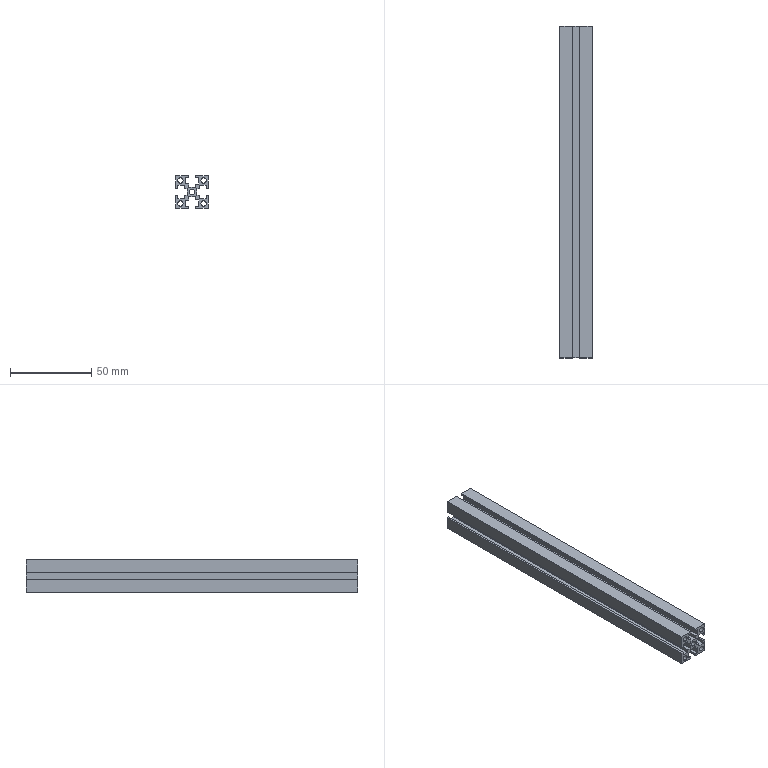Part | STEP file | 20 aluminium profile longitudinal 6 | 1 solid | 64 faces | box 20 x 204 x 20 mm | volume 36267 mm3 | plane 54 | cylinder 10 | commonest cylinder face diameters 3.3 x10